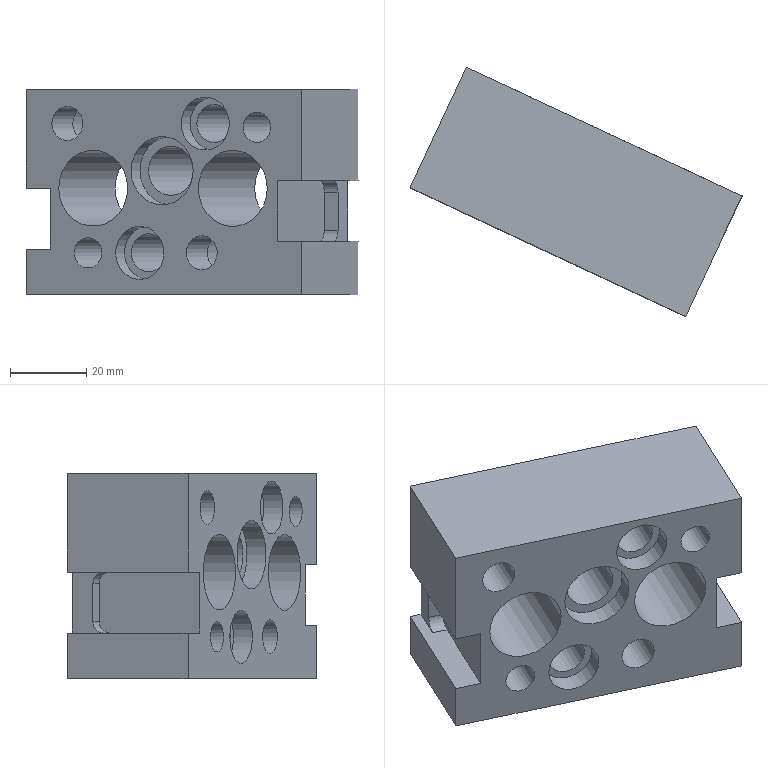Part | STEP file | gslz 2016.10.28-13_id446_x_t | 1 solid | 41 faces | box 87.296 x 65.53 x 54 mm | volume 98579 mm3 | plane 23 | cylinder 18 | commonest cylinder face diameters 6 x4 14 x4 8 x2 9 x2 10 x2 20 x2